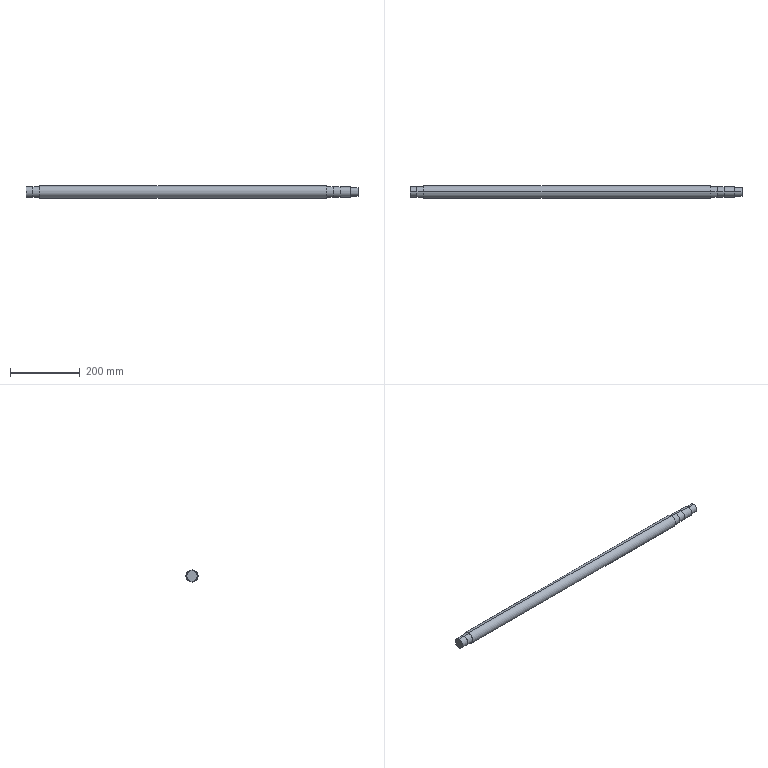Part | SolidWorks | features ICE 6, Extrusion 1, HoleWzd 1, MirrorPattern 1 | 1 solid | 41 faces | box 949 x 35 x 35 mm | volume 873181 mm3 | cylinder 22 | plane 17 | cone 2 | commonest cylinder face diameters 10 x4 30 x4 31 x4 6.8 x2 8 x2 25 x2
STEP:
#1=CARTESIAN_POINT('',(480.,0.,3.4));
#2=VERTEX_POINT('',#1);
#3=CARTESIAN_POINT('',(480.,0.,-3.4));
#4=VERTEX_POINT('',#3);
#5=CARTESIAN_POINT('',(480.,0.,0.));
#6=DIRECTION('',(1.,0.,0.));
#7=DIRECTION('',(0.,0.,-1.));
#8=AXIS2_PLACEMENT_3D('',#5,#6,#7);
#9=CIRCLE('',#8,3.4);
#10=EDGE_CURVE('',#2,#4,#9,.T.);
#11=ORIENTED_EDGE('',*,*,#10,.F.);
#12=CARTESIAN_POINT('',(500.,0.,3.4));
#13=VERTEX_POINT('',#12);
#14=CARTESIAN_POINT('',(500.,0.,3.4));
#15=DIRECTION('',(1.,0.,0.));
#16=VECTOR('',#15,1000.);
#17=LINE('',#14,#16);
#18=EDGE_CURVE('',#2,#13,#17,.T.);
#19=ORIENTED_EDGE('',*,*,#18,.T.);
#20=CARTESIAN_POINT('',(500.,0.,-3.4));
#21=VERTEX_POINT('',#20);
#22=CARTESIAN_POINT('',(500.,0.,0.));
#23=DIRECTION('',(1.,0.,0.));
#24=DIRECTION('',(0.,0.,-1.));
#25=AXIS2_PLACEMENT_3D('',#22,#23,#24);
#26=CIRCLE('',#25,3.4);
#27=EDGE_CURVE('',#13,#21,#26,.T.);
#28=ORIENTED_EDGE('',*,*,#27,.T.);
#29=CARTESIAN_POINT('',(500.,0.,-3.4));
#30=DIRECTION('',(1.,0.,0.));
#31=VECTOR('',#30,1000.);
#32=LINE('',#29,#31);
#33=EDGE_CURVE('',#4,#21,#32,.T.);
#34=ORIENTED_EDGE('',*,*,#33,.F.);
#35=EDGE_LOOP('',(#11,#19,#28,#34));
#36=FACE_OUTER_BOUND('',#35,.T.);
#37=CARTESIAN_POINT('',(500.,0.,0.));
#38=DIRECTION('',(1.,0.,0.));
#39=DIRECTION('',(0.,0.,-1.));
#40=AXIS2_PLACEMENT_3D('',#37,#38,#39);
#41=CYLINDRICAL_SURFACE('',#40,3.4);
#42=ADVANCED_FACE('',(#36),#41,.F.);
#43=CARTESIAN_POINT('',(477.957,0.,0.));
#44=VERTEX_POINT('',#43);
#45=CARTESIAN_POINT('',(480.,0.,-3.4));
#46=DIRECTION('',(0.515,0.,-0.8572));
#47=VECTOR('',#46,1000.);
#48=LINE('',#45,#47);
#49=EDGE_CURVE('',#44,#4,#48,.T.);
#50=ORIENTED_EDGE('',*,*,#49,.F.);
#51=CARTESIAN_POINT('',(480.,0.,3.4));
#52=DIRECTION('',(0.515,0.,0.8572));
#53=VECTOR('',#52,1000.);
#54=LINE('',#51,#53);
#55=EDGE_CURVE('',#44,#2,#54,.T.);
#56=ORIENTED_EDGE('',*,*,#55,.T.);
#57=ORIENTED_EDGE('',*,*,#10,.T.);
#58=EDGE_LOOP('',(#50,#56,#57));
#59=FACE_OUTER_BOUND('',#58,.T.);
#60=CARTESIAN_POINT('',(480.,0.,0.));
#61=DIRECTION('',(1.,0.,0.));
#62=DIRECTION('',(0.,0.,-1.));
#63=AXIS2_PLACEMENT_3D('',#60,#61,#62);
#64=CONICAL_SURFACE('',#63,3.4,1.03);
#65=ADVANCED_FACE('',(#59),#64,.F.);
#66=CARTESIAN_POINT('',(-449.,0.,-15.));
#67=VERTEX_POINT('',#66);
#68=CARTESIAN_POINT('',(-449.,0.,15.));
#69=VERTEX_POINT('',#68);
#70=CARTESIAN_POINT('',(-449.,0.,0.));
#71=DIRECTION('',(1.,0.,0.));
#72=DIRECTION('',(0.,0.,-1.));
#73=AXIS2_PLACEMENT_3D('',#70,#71,#72);
#74=CIRCLE('',#73,15.);
#75=EDGE_CURVE('',#67,#69,#74,.T.);
#76=ORIENTED_EDGE('',*,*,#75,.T.);
#77=CARTESIAN_POINT('',(-429.,0.,15.));
#78=VERTEX_POINT('',#77);
#79=CARTESIAN_POINT('',(-449.,0.,15.));
#80=DIRECTION('',(1.,0.,0.));
#81=VECTOR('',#80,1000.);
#82=LINE('',#79,#81);
#83=EDGE_CURVE('',#69,#78,#82,.T.);
#84=ORIENTED_EDGE('',*,*,#83,.T.);
#85=CARTESIAN_POINT('',(-429.,0.,-15.));
#86=VERTEX_POINT('',#85);
#87=CARTESIAN_POINT('',(-429.,0.,0.));
#88=DIRECTION('',(-1.,0.,0.));
#89=DIRECTION('',(0.,0.,1.));
#90=AXIS2_PLACEMENT_3D('',#87,#88,#89);
#91=CIRCLE('',#90,15.);
#92=EDGE_CURVE('',#78,#86,#91,.T.);
#93=ORIENTED_EDGE('',*,*,#92,.T.);
#94=CARTESIAN_POINT('',(-449.,0.,-15.));
#95=DIRECTION('',(1.,0.,0.));
#96=VECTOR('',#95,1000.);
#97=LINE('',#94,#96);
#98=EDGE_CURVE('',#67,#86,#97,.T.);
#99=ORIENTED_EDGE('',*,*,#98,.F.);
#100=EDGE_LOOP('',(#76,#84,#93,#99));
#101=FACE_OUTER_BOUND('',#100,.T.);
#102=CARTESIAN_POINT('',(-449.,0.,0.));
#103=DIRECTION('',(1.,0.,0.));
#104=DIRECTION('',(0.,0.,-1.));
#105=AXIS2_PLACEMENT_3D('',#102,#103,#104);
#106=CYLINDRICAL_SURFACE('',#105,15.);
#107=ADVANCED_FACE('',(#101),#106,.T.);
#108=CARTESIAN_POINT('',(-422.,14.671,-5.));
#109=VERTEX_POINT('',#108);
#110=CARTESIAN_POINT('',(-422.,14.671,5.));
#111=VERTEX_POINT('',#110);
#112=CARTESIAN_POINT('',(-422.,14.671,-5.));
#113=CARTESIAN_POINT('',(-422.333,14.671,-5.));
#114=CARTESIAN_POINT('',(-422.659,14.683,-4.967));
#115=CARTESIAN_POINT('',(-423.301,14.725,-4.839));
#116=CARTESIAN_POINT('',(-423.62,14.757,-4.742));
#117=CARTESIAN_POINT('',(-424.224,14.836,-4.49));
#118=CARTESIAN_POINT('',(-424.51,14.882,-4.337));
#119=CARTESIAN_POINT('',(-425.052,14.983,-3.974));
#120=CARTESIAN_POINT('',(-425.306,15.038,-3.765));
#121=CARTESIAN_POINT('',(-425.764,15.145,-3.307));
#122=CARTESIAN_POINT('',(-425.97,15.198,-3.057));
#123=CARTESIAN_POINT('',(-426.336,15.298,-2.511));
#124=CARTESIAN_POINT('',(-426.49,15.343,-2.224));
#125=CARTESIAN_POINT('',(-426.678,15.399,-1.773));
#126=CARTESIAN_POINT('',(-426.733,15.416,-1.62));
#127=CARTESIAN_POINT('',(-426.829,15.446,-1.306));
#128=CARTESIAN_POINT('',(-426.87,15.459,-1.144));
#129=CARTESIAN_POINT('',(-426.967,15.489,-0.6596));
#130=CARTESIAN_POINT('',(-427.,15.5,-0.3337));
#131=CARTESIAN_POINT('',(-427.,15.5,0.3234));
#132=CARTESIAN_POINT('',(-426.967,15.489,0.6571));
#133=CARTESIAN_POINT('',(-426.839,15.449,1.3));
#134=CARTESIAN_POINT('',(-426.744,15.419,1.613));
#135=CARTESIAN_POINT('',(-426.492,15.343,2.221));
#136=CARTESIAN_POINT('',(-426.336,15.298,2.51));
#137=CARTESIAN_POINT('',(-425.975,15.199,3.05));
#138=CARTESIAN_POINT('',(-425.767,15.146,3.304));
#139=CARTESIAN_POINT('',(-425.306,15.038,3.765));
#140=CARTESIAN_POINT('',(-425.056,14.984,3.97));
#141=CARTESIAN_POINT('',(-424.517,14.883,4.333));
#142=CARTESIAN_POINT('',(-424.225,14.836,4.49));
#143=CARTESIAN_POINT('',(-423.623,14.758,4.74));
#144=CARTESIAN_POINT('',(-423.311,14.726,4.836));
#145=CARTESIAN_POINT('',(-422.665,14.683,4.967));
#146=CARTESIAN_POINT('',(-422.333,14.671,5.));
#147=CARTESIAN_POINT('',(-422.,14.671,5.));
#148=B_SPLINE_CURVE_WITH_KNOTS('',3,(#112,#113,#114,#115,#116,#117,#118,#119,#120,#121,#122,#123,#124,#125,#126,#127,#128,#129,#130,#131,#132,#133,#134,#135,#136,#137,#138,#139,#140,#141,#142,#143,#144,#145,#146,#147),.UNSPECIFIED.,.F.,.F.,(4,2,2,2,2,2,2,2,2,2,2,2,2,2,2,2,2,4),(0.,0.0009833,0.001967,0.00295,0.003933,0.004916,0.0059,0.006391,0.006883,0.007866,0.008849,0.009833,0.01082,0.0118,0.01278,0.01377,0.01475,0.01573),.UNSPECIFIED.);
#149=EDGE_CURVE('',#109,#111,#148,.T.);
#150=ORIENTED_EDGE('',*,*,#149,.F.);
#151=CARTESIAN_POINT('',(-418.,14.671,-5.));
#152=VERTEX_POINT('',#151);
#153=CARTESIAN_POINT('',(-429.,14.671,-5.));
#154=DIRECTION('',(-1.,0.,0.));
#155=VECTOR('',#154,1000.);
#156=LINE('',#153,#155);
#157=EDGE_CURVE('',#152,#109,#156,.T.);
#158=ORIENTED_EDGE('',*,*,#157,.F.);
#159=CARTESIAN_POINT('',(-418.,14.671,5.));
#160=VERTEX_POINT('',#159);
#161=CARTESIAN_POINT('',(-418.,14.671,5.));
#162=CARTESIAN_POINT('',(-417.667,14.671,5.));
#163=CARTESIAN_POINT('',(-417.34,14.683,4.967));
#164=CARTESIAN_POINT('',(-416.698,14.726,4.839));
#165=CARTESIAN_POINT('',(-416.38,14.758,4.741));
#166=CARTESIAN_POINT('',(-415.775,14.836,4.49));
#167=CARTESIAN_POINT('',(-415.489,14.882,4.336));
#168=CARTESIAN_POINT('',(-414.947,14.983,3.973));
#169=CARTESIAN_POINT('',(-414.693,15.038,3.764));
#170=CARTESIAN_POINT('',(-414.235,15.145,3.306));
#171=CARTESIAN_POINT('',(-414.029,15.198,3.056));
#172=CARTESIAN_POINT('',(-413.663,15.298,2.509));
#173=CARTESIAN_POINT('',(-413.509,15.343,2.222));
#174=CARTESIAN_POINT('',(-413.321,15.399,1.771));
#175=CARTESIAN_POINT('',(-413.266,15.416,1.618));
#176=CARTESIAN_POINT('',(-413.17,15.446,1.303));
#177=CARTESIAN_POINT('',(-413.129,15.459,1.142));
#178=CARTESIAN_POINT('',(-413.032,15.489,0.6569));
#179=CARTESIAN_POINT('',(-413.,15.5,0.3309));
#180=CARTESIAN_POINT('',(-413.,15.5,-0.3264));
#181=CARTESIAN_POINT('',(-413.033,15.489,-0.6603));
#182=CARTESIAN_POINT('',(-413.162,15.448,-1.304));
#183=CARTESIAN_POINT('',(-413.257,15.419,-1.616));
#184=CARTESIAN_POINT('',(-413.51,15.343,-2.225));
#185=CARTESIAN_POINT('',(-413.666,15.297,-2.514));
#186=CARTESIAN_POINT('',(-414.027,15.199,-3.053));
#187=CARTESIAN_POINT('',(-414.236,15.145,-3.307));
#188=CARTESIAN_POINT('',(-414.697,15.037,-3.768));
#189=CARTESIAN_POINT('',(-414.947,14.983,-3.973));
#190=CARTESIAN_POINT('',(-415.487,14.883,-4.335));
#191=CARTESIAN_POINT('',(-415.78,14.835,-4.492));
#192=CARTESIAN_POINT('',(-416.382,14.757,-4.742));
#193=CARTESIAN_POINT('',(-416.694,14.726,-4.838));
#194=CARTESIAN_POINT('',(-417.179,14.693,-4.935));
#195=CARTESIAN_POINT('',(-417.344,14.685,-4.96));
#196=CARTESIAN_POINT('',(-417.672,14.674,-4.992));
#197=CARTESIAN_POINT('',(-417.836,14.671,-5.));
#198=CARTESIAN_POINT('',(-418.,14.671,-5.));
#199=B_SPLINE_CURVE_WITH_KNOTS('',3,(#161,#162,#163,#164,#165,#166,#167,#168,#169,#170,#171,#172,#173,#174,#175,#176,#177,#178,#179,#180,#181,#182,#183,#184,#185,#186,#187,#188,#189,#190,#191,#192,#193,#194,#195,#196,#197,#198),.UNSPECIFIED.,.F.,.F.,(4,2,2,2,2,2,2,2,2,2,2,2,2,2,2,2,2,2,4),(0.,0.0009836,0.001967,0.002951,0.003934,0.004918,0.005902,0.006394,0.006885,0.007869,0.008853,0.009836,0.01082,0.0118,0.01279,0.01377,0.01475,0.01525,0.01574),.UNSPECIFIED.);
#200=EDGE_CURVE('',#160,#152,#199,.T.);
#201=ORIENTED_EDGE('',*,*,#200,.F.);
#202=CARTESIAN_POINT('',(-429.,14.671,5.));
#203=DIRECTION('',(1.,0.,0.));
#204=VECTOR('',#203,1000.);
#205=LINE('',#202,#204);
#206=EDGE_CURVE('',#111,#160,#205,.T.);
#207=ORIENTED_EDGE('',*,*,#206,.F.);
#208=EDGE_LOOP('',(#150,#158,#201,#207));
#209=FACE_BOUND('',#208,.T.);
#210=CARTESIAN_POINT('',(-429.,0.,-15.5));
#211=VERTEX_POINT('',#210);
#212=CARTESIAN_POINT('',(-429.,0.,15.5));
#213=VERTEX_POINT('',#212);
#214=CARTESIAN_POINT('',(-429.,0.,0.));
#215=DIRECTION('',(1.,0.,0.));
#216=DIRECTION('',(0.,0.,-1.));
#217=AXIS2_PLACEMENT_3D('',#214,#215,#216);
#218=CIRCLE('',#217,15.5);
#219=EDGE_CURVE('',#211,#213,#218,.T.);
#220=ORIENTED_EDGE('',*,*,#219,.T.);
#221=CARTESIAN_POINT('',(-410.,0.,15.5));
#222=VERTEX_POINT('',#221);
#223=CARTESIAN_POINT('',(-429.,0.,15.5));
#224=DIRECTION('',(1.,0.,0.));
#225=VECTOR('',#224,1000.);
#226=LINE('',#223,#225);
#227=EDGE_CURVE('',#213,#222,#226,.T.);
#228=ORIENTED_EDGE('',*,*,#227,.T.);
#229=CARTESIAN_POINT('',(-410.,0.,-15.5));
#230=VERTEX_POINT('',#229);
#231=CARTESIAN_POINT('',(-410.,0.,0.));
#232=DIRECTION('',(1.,0.,0.));
#233=DIRECTION('',(0.,0.,-1.));
#234=AXIS2_PLACEMENT_3D('',#231,#232,#233);
#235=CIRCLE('',#234,15.5);
#236=EDGE_CURVE('',#230,#222,#235,.T.);
#237=ORIENTED_EDGE('',*,*,#236,.F.);
#238=CARTESIAN_POINT('',(-429.,0.,-15.5));
#239=DIRECTION('',(1.,0.,0.));
#240=VECTOR('',#239,1000.);
#241=LINE('',#238,#240);
#242=EDGE_CURVE('',#211,#230,#241,.T.);
#243=ORIENTED_EDGE('',*,*,#242,.F.);
#244=EDGE_LOOP('',(#220,#228,#237,#243));
#245=FACE_OUTER_BOUND('',#244,.T.);
#246=CARTESIAN_POINT('',(-429.,0.,0.));
#247=DIRECTION('',(1.,0.,0.));
#248=DIRECTION('',(0.,0.,-1.));
#249=AXIS2_PLACEMENT_3D('',#246,#247,#248);
#250=CYLINDRICAL_SURFACE('',#249,15.5);
#251=ADVANCED_FACE('',(#209,#245),#250,.T.);
#252=CARTESIAN_POINT('',(494.,11.843,4.));
#253=VERTEX_POINT('',#252);
#254=CARTESIAN_POINT('',(484.,11.843,4.));
#255=VERTEX_POINT('',#254);
#256=CARTESIAN_POINT('',(500.,11.843,4.));
#257=DIRECTION('',(-1.,0.,0.));
#258=VECTOR('',#257,1000.);
#259=LINE('',#256,#258);
#260=EDGE_CURVE('',#253,#255,#259,.T.);
#261=ORIENTED_EDGE('',*,*,#260,.T.);
#262=CARTESIAN_POINT('',(484.,11.843,-4.));
#263=VERTEX_POINT('',#262);
#264=CARTESIAN_POINT('',(484.,11.843,4.));
#265=CARTESIAN_POINT('',(483.734,11.843,4.));
#266=CARTESIAN_POINT('',(483.473,11.852,3.974));
#267=CARTESIAN_POINT('',(482.959,11.886,3.871));
#268=CARTESIAN_POINT('',(482.704,11.911,3.793));
#269=CARTESIAN_POINT('',(482.221,11.973,3.592));
#270=CARTESIAN_POINT('',(481.992,12.01,3.469));
#271=CARTESIAN_POINT('',(481.559,12.09,3.179));
#272=CARTESIAN_POINT('',(481.355,12.133,3.012));
#273=CARTESIAN_POINT('',(480.989,12.218,2.646));
#274=CARTESIAN_POINT('',(480.824,12.26,2.445));
#275=CARTESIAN_POINT('',(480.531,12.34,2.009));
#276=CARTESIAN_POINT('',(480.408,12.375,1.779));
#277=CARTESIAN_POINT('',(480.208,12.435,1.299));
#278=CARTESIAN_POINT('',(480.13,12.459,1.045));
#279=CARTESIAN_POINT('',(480.026,12.492,0.5276));
#280=CARTESIAN_POINT('',(480.,12.5,0.2669));
#281=CARTESIAN_POINT('',(480.,12.5,-0.2587));
#282=CARTESIAN_POINT('',(480.026,12.492,-0.5256));
#283=CARTESIAN_POINT('',(480.129,12.459,-1.04));
#284=CARTESIAN_POINT('',(480.205,12.436,-1.29));
#285=CARTESIAN_POINT('',(480.407,12.375,-1.777));
#286=CARTESIAN_POINT('',(480.531,12.34,-2.008));
#287=CARTESIAN_POINT('',(480.82,12.262,-2.44));
#288=CARTESIAN_POINT('',(480.987,12.219,-2.643));
#289=CARTESIAN_POINT('',(481.355,12.133,-3.012));
#290=CARTESIAN_POINT('',(481.555,12.091,-3.176));
#291=CARTESIAN_POINT('',(481.987,12.011,-3.466));
#292=CARTESIAN_POINT('',(482.22,11.973,-3.592));
#293=CARTESIAN_POINT('',(482.702,11.911,-3.792));
#294=CARTESIAN_POINT('',(482.951,11.886,-3.869));
#295=CARTESIAN_POINT('',(483.468,11.852,-3.973));
#296=CARTESIAN_POINT('',(483.734,11.843,-4.));
#297=CARTESIAN_POINT('',(484.,11.843,-4.));
#298=B_SPLINE_CURVE_WITH_KNOTS('',3,(#264,#265,#266,#267,#268,#269,#270,#271,#272,#273,#274,#275,#276,#277,#278,#279,#280,#281,#282,#283,#284,#285,#286,#287,#288,#289,#290,#291,#292,#293,#294,#295,#296,#297),.UNSPECIFIED.,.F.,.F.,(4,2,2,2,2,2,2,2,2,2,2,2,2,2,2,2,4),(0.,0.0007865,0.001573,0.00236,0.003146,0.003933,0.004719,0.005506,0.006292,0.007079,0.007865,0.008652,0.009438,0.01022,0.01101,0.0118,0.01258),.UNSPECIFIED.);
#299=EDGE_CURVE('',#255,#263,#298,.T.);
#300=ORIENTED_EDGE('',*,*,#299,.T.);
#301=CARTESIAN_POINT('',(494.,11.843,-4.));
#302=VERTEX_POINT('',#301);
#303=CARTESIAN_POINT('',(500.,11.843,-4.));
#304=DIRECTION('',(1.,0.,0.));
#305=VECTOR('',#304,1000.);
#306=LINE('',#303,#305);
#307=EDGE_CURVE('',#263,#302,#306,.T.);
#308=ORIENTED_EDGE('',*,*,#307,.T.);
#309=CARTESIAN_POINT('',(494.,11.843,-4.));
#310=CARTESIAN_POINT('',(494.266,11.843,-4.));
#311=CARTESIAN_POINT('',(494.527,11.852,-3.974));
#312=CARTESIAN_POINT('',(495.041,11.886,-3.871));
#313=CARTESIAN_POINT('',(495.296,11.911,-3.793));
#314=CARTESIAN_POINT('',(495.779,11.973,-3.592));
#315=CARTESIAN_POINT('',(496.008,12.01,-3.469));
#316=CARTESIAN_POINT('',(496.441,12.09,-3.179));
#317=CARTESIAN_POINT('',(496.645,12.133,-3.012));
#318=CARTESIAN_POINT('',(497.011,12.218,-2.646));
#319=CARTESIAN_POINT('',(497.176,12.26,-2.445));
#320=CARTESIAN_POINT('',(497.469,12.34,-2.009));
#321=CARTESIAN_POINT('',(497.592,12.375,-1.779));
#322=CARTESIAN_POINT('',(497.792,12.435,-1.299));
#323=CARTESIAN_POINT('',(497.87,12.459,-1.045));
#324=CARTESIAN_POINT('',(497.974,12.492,-0.5276));
#325=CARTESIAN_POINT('',(498.,12.5,-0.2669));
#326=CARTESIAN_POINT('',(498.,12.5,0.2587));
#327=CARTESIAN_POINT('',(497.974,12.492,0.5256));
#328=CARTESIAN_POINT('',(497.871,12.459,1.04));
#329=CARTESIAN_POINT('',(497.795,12.436,1.29));
#330=CARTESIAN_POINT('',(497.593,12.375,1.777));
#331=CARTESIAN_POINT('',(497.469,12.34,2.008));
#332=CARTESIAN_POINT('',(497.18,12.262,2.44));
#333=CARTESIAN_POINT('',(497.013,12.219,2.643));
#334=CARTESIAN_POINT('',(496.645,12.133,3.012));
#335=CARTESIAN_POINT('',(496.445,12.091,3.176));
#336=CARTESIAN_POINT('',(496.013,12.011,3.466));
#337=CARTESIAN_POINT('',(495.78,11.973,3.592));
#338=CARTESIAN_POINT('',(495.298,11.911,3.792));
#339=CARTESIAN_POINT('',(495.049,11.886,3.869));
#340=CARTESIAN_POINT('',(494.532,11.852,3.973));
#341=CARTESIAN_POINT('',(494.266,11.843,4.));
#342=CARTESIAN_POINT('',(494.,11.843,4.));
#343=B_SPLINE_CURVE_WITH_KNOTS('',3,(#309,#310,#311,#312,#313,#314,#315,#316,#317,#318,#319,#320,#321,#322,#323,#324,#325,#326,#327,#328,#329,#330,#331,#332,#333,#334,#335,#336,#337,#338,#339,#340,#341,#342),.UNSPECIFIED.,.F.,.F.,(4,2,2,2,2,2,2,2,2,2,2,2,2,2,2,2,4),(0.,0.0007865,0.001573,0.00236,0.003146,0.003933,0.004719,0.005506,0.006292,0.007079,0.007865,0.008652,0.009438,0.01022,0.01101,0.0118,0.01258),.UNSPECIFIED.);
#344=EDGE_CURVE('',#302,#253,#343,.T.);
#345=ORIENTED_EDGE('',*,*,#344,.T.);
#346=EDGE_LOOP('',(#261,#300,#308,#345));
#347=FACE_BOUND('',#346,.T.);
#348=CARTESIAN_POINT('',(500.,0.,-12.5));
#349=VERTEX_POINT('',#348);
#350=CARTESIAN_POINT('',(500.,0.,12.5));
#351=VERTEX_POINT('',#350);
#352=CARTESIAN_POINT('',(500.,0.,0.));
#353=DIRECTION('',(1.,0.,0.));
#354=DIRECTION('',(0.,0.,-1.));
#355=AXIS2_PLACEMENT_3D('',#352,#353,#354);
#356=CIRCLE('',#355,12.5);
#357=EDGE_CURVE('',#349,#351,#356,.T.);
#358=ORIENTED_EDGE('',*,*,#357,.F.);
#359=CARTESIAN_POINT('',(478.,0.,-12.5));
#360=VERTEX_POINT('',#359);
#361=CARTESIAN_POINT('',(500.,0.,-12.5));
#362=DIRECTION('',(-1.,0.,0.));
#363=VECTOR('',#362,1000.);
#364=LINE('',#361,#363);
#365=EDGE_CURVE('',#349,#360,#364,.T.);
#366=ORIENTED_EDGE('',*,*,#365,.T.);
#367=CARTESIAN_POINT('',(478.,0.,12.5));
#368=VERTEX_POINT('',#367);
#369=CARTESIAN_POINT('',(478.,0.,0.));
#370=DIRECTION('',(1.,0.,0.));
#371=DIRECTION('',(0.,0.,-1.));
#372=AXIS2_PLACEMENT_3D('',#369,#370,#371);
#373=CIRCLE('',#372,12.5);
#374=EDGE_CURVE('',#360,#368,#373,.T.);
#375=ORIENTED_EDGE('',*,*,#374,.T.);
#376=CARTESIAN_POINT('',(500.,0.,12.5));
#377=DIRECTION('',(-1.,0.,0.));
#378=VECTOR('',#377,1000.);
#379=LINE('',#376,#378);
#380=EDGE_CURVE('',#351,#368,#379,.T.);
#381=ORIENTED_EDGE('',*,*,#380,.F.);
#382=EDGE_LOOP('',(#358,#366,#375,#381));
#383=FACE_OUTER_BOUND('',#382,.T.);
#384=CARTESIAN_POINT('',(500.,0.,0.));
#385=DIRECTION('',(-1.,0.,0.));
#386=DIRECTION('',(0.,0.,1.));
#387=AXIS2_PLACEMENT_3D('',#384,#385,#386);
#388=CYLINDRICAL_SURFACE('',#387,12.5);
#389=ADVANCED_FACE('',(#347,#383),#388,.T.);
#390=CARTESIAN_POINT('',(478.,0.,-14.5));
#391=VERTEX_POINT('',#390);
#392=CARTESIAN_POINT('',(478.,0.,14.5));
#393=VERTEX_POINT('',#392);
#394=CARTESIAN_POINT('',(478.,0.,0.));
#395=DIRECTION('',(1.,0.,0.));
#396=DIRECTION('',(0.,0.,-1.));
#397=AXIS2_PLACEMENT_3D('',#394,#395,#396);
#398=CIRCLE('',#397,14.5);
#399=EDGE_CURVE('',#391,#393,#398,.T.);
#400=ORIENTED_EDGE('',*,*,#399,.F.);
#401=CARTESIAN_POINT('',(449.,0.,-14.5));
#402=VERTEX_POINT('',#401);
#403=CARTESIAN_POINT('',(478.,0.,-14.5));
#404=DIRECTION('',(-1.,0.,0.));
#405=VECTOR('',#404,1000.);
#406=LINE('',#403,#405);
#407=EDGE_CURVE('',#391,#402,#406,.T.);
#408=ORIENTED_EDGE('',*,*,#407,.T.);
#409=CARTESIAN_POINT('',(449.,0.,14.5));
#410=VERTEX_POINT('',#409);
#411=CARTESIAN_POINT('',(449.,0.,0.));
#412=DIRECTION('',(1.,0.,0.));
#413=DIRECTION('',(0.,0.,-1.));
#414=AXIS2_PLACEMENT_3D('',#411,#412,#413);
#415=CIRCLE('',#414,14.5);
#416=EDGE_CURVE('',#402,#410,#415,.T.);
#417=ORIENTED_EDGE('',*,*,#416,.T.);
#418=CARTESIAN_POINT('',(478.,0.,14.5));
#419=DIRECTION('',(-1.,0.,0.));
#420=VECTOR('',#419,1000.);
#421=LINE('',#418,#420);
#422=EDGE_CURVE('',#393,#410,#421,.T.);
#423=ORIENTED_EDGE('',*,*,#422,.F.);
#424=EDGE_LOOP('',(#400,#408,#417,#423));
#425=FACE_OUTER_BOUND('',#424,.T.);
#426=CARTESIAN_POINT('',(478.,0.,0.));
#427=DIRECTION('',(-1.,0.,0.));
#428=DIRECTION('',(0.,0.,1.));
#429=AXIS2_PLACEMENT_3D('',#426,#427,#428);
#430=CYLINDRICAL_SURFACE('',#429,14.5);
#431=ADVANCED_FACE('',(#425),#430,.T.);
#432=CARTESIAN_POINT('',(449.,0.,-15.));
#433=VERTEX_POINT('',#432);
#434=CARTESIAN_POINT('',(449.,0.,15.));
#435=VERTEX_POINT('',#434);
#436=CARTESIAN_POINT('',(449.,0.,0.));
#437=DIRECTION('',(1.,0.,0.));
#438=DIRECTION('',(0.,0.,-1.));
#439=AXIS2_PLACEMENT_3D('',#436,#437,#438);
#440=CIRCLE('',#439,15.);
#441=EDGE_CURVE('',#433,#435,#440,.T.);
#442=ORIENTED_EDGE('',*,*,#441,.F.);
#443=CARTESIAN_POINT('',(429.,0.,-15.));
#444=VERTEX_POINT('',#443);
#445=CARTESIAN_POINT('',(449.,0.,-15.));
#446=DIRECTION('',(-1.,0.,0.));
#447=VECTOR('',#446,1000.);
#448=LINE('',#445,#447);
#449=EDGE_CURVE('',#433,#444,#448,.T.);
#450=ORIENTED_EDGE('',*,*,#449,.T.);
#451=CARTESIAN_POINT('',(429.,0.,15.));
#452=VERTEX_POINT('',#451);
#453=CARTESIAN_POINT('',(429.,0.,0.));
#454=DIRECTION('',(1.,0.,0.));
#455=DIRECTION('',(0.,0.,-1.));
#456=AXIS2_PLACEMENT_3D('',#453,#454,#455);
#457=CIRCLE('',#456,15.);
#458=EDGE_CURVE('',#444,#452,#457,.T.);
#459=ORIENTED_EDGE('',*,*,#458,.T.);
#460=CARTESIAN_POINT('',(449.,0.,15.));
#461=DIRECTION('',(-1.,0.,0.));
#462=VECTOR('',#461,1000.);
#463=LINE('',#460,#462);
#464=EDGE_CURVE('',#435,#452,#463,.T.);
#465=ORIENTED_EDGE('',*,*,#464,.F.);
#466=EDGE_LOOP('',(#442,#450,#459,#465));
#467=FACE_OUTER_BOUND('',#466,.T.);
#468=CARTESIAN_POINT('',(449.,0.,0.));
#469=DIRECTION('',(-1.,0.,0.));
#470=DIRECTION('',(0.,0.,1.));
#471=AXIS2_PLACEMENT_3D('',#468,#469,#470);
#472=CYLINDRICAL_SURFACE('',#471,15.);
#473=ADVANCED_FACE('',(#467),#472,.T.);
#474=CARTESIAN_POINT('',(422.,14.671,5.));
#475=VERTEX_POINT('',#474);
#476=CARTESIAN_POINT('',(418.,14.671,5.));
#477=VERTEX_POINT('',#476);
#478=CARTESIAN_POINT('',(429.,14.671,5.));
#479=DIRECTION('',(-1.,0.,0.));
#480=VECTOR('',#479,1000.);
#481=LINE('',#478,#480);
#482=EDGE_CURVE('',#475,#477,#481,.T.);
#483=ORIENTED_EDGE('',*,*,#482,.T.);
#484=CARTESIAN_POINT('',(418.,14.671,-5.));
#485=VERTEX_POINT('',#484);
#486=CARTESIAN_POINT('',(418.,14.671,5.));
#487=CARTESIAN_POINT('',(417.667,14.671,5.));
#488=CARTESIAN_POINT('',(417.341,14.683,4.967));
#489=CARTESIAN_POINT('',(416.699,14.725,4.839));
#490=CARTESIAN_POINT('',(416.38,14.757,4.742));
#491=CARTESIAN_POINT('',(415.776,14.836,4.49));
#492=CARTESIAN_POINT('',(415.49,14.882,4.337));
#493=CARTESIAN_POINT('',(414.948,14.983,3.974));
#494=CARTESIAN_POINT('',(414.694,15.038,3.765));
#495=CARTESIAN_POINT('',(414.236,15.145,3.307));
#496=CARTESIAN_POINT('',(414.03,15.198,3.057));
#497=CARTESIAN_POINT('',(413.664,15.298,2.511));
#498=CARTESIAN_POINT('',(413.51,15.343,2.224));
#499=CARTESIAN_POINT('',(413.322,15.399,1.773));
#500=CARTESIAN_POINT('',(413.267,15.416,1.62));
#501=CARTESIAN_POINT('',(413.171,15.446,1.306));
#502=CARTESIAN_POINT('',(413.13,15.459,1.144));
#503=CARTESIAN_POINT('',(413.033,15.489,0.6596));
#504=CARTESIAN_POINT('',(413.,15.5,0.3337));
#505=CARTESIAN_POINT('',(413.,15.5,-0.3234));
#506=CARTESIAN_POINT('',(413.033,15.489,-0.6571));
#507=CARTESIAN_POINT('',(413.161,15.449,-1.3));
#508=CARTESIAN_POINT('',(413.256,15.419,-1.613));
#509=CARTESIAN_POINT('',(413.508,15.343,-2.221));
#510=CARTESIAN_POINT('',(413.664,15.298,-2.51));
#511=CARTESIAN_POINT('',(414.025,15.199,-3.05));
#512=CARTESIAN_POINT('',(414.233,15.146,-3.304));
#513=CARTESIAN_POINT('',(414.694,15.038,-3.765));
#514=CARTESIAN_POINT('',(414.944,14.984,-3.97));
#515=CARTESIAN_POINT('',(415.483,14.883,-4.333));
#516=CARTESIAN_POINT('',(415.775,14.836,-4.49));
#517=CARTESIAN_POINT('',(416.377,14.758,-4.74));
#518=CARTESIAN_POINT('',(416.689,14.726,-4.836));
#519=CARTESIAN_POINT('',(417.335,14.683,-4.967));
#520=CARTESIAN_POINT('',(417.667,14.671,-5.));
#521=CARTESIAN_POINT('',(418.,14.671,-5.));
#522=B_SPLINE_CURVE_WITH_KNOTS('',3,(#486,#487,#488,#489,#490,#491,#492,#493,#494,#495,#496,#497,#498,#499,#500,#501,#502,#503,#504,#505,#506,#507,#508,#509,#510,#511,#512,#513,#514,#515,#516,#517,#518,#519,#520,#521),.UNSPECIFIED.,.F.,.F.,(4,2,2,2,2,2,2,2,2,2,2,2,2,2,2,2,2,4),(0.,0.0009833,0.001967,0.00295,0.003933,0.004916,0.0059,0.006391,0.006883,0.007866,0.008849,0.009833,0.01082,0.0118,0.01278,0.01377,0.01475,0.01573),.UNSPECIFIED.);
#523=EDGE_CURVE('',#477,#485,#522,.T.);
#524=ORIENTED_EDGE('',*,*,#523,.T.);
#525=CARTESIAN_POINT('',(422.,14.671,-5.));
#526=VERTEX_POINT('',#525);
#527=CARTESIAN_POINT('',(429.,14.671,-5.));
#528=DIRECTION('',(1.,0.,0.));
#529=VECTOR('',#528,1000.);
#530=LINE('',#527,#529);
#531=EDGE_CURVE('',#485,#526,#530,.T.);
#532=ORIENTED_EDGE('',*,*,#531,.T.);
#533=CARTESIAN_POINT('',(422.,14.671,-5.));
#534=CARTESIAN_POINT('',(422.328,14.671,-5.));
#535=CARTESIAN_POINT('',(422.657,14.683,-4.968));
#536=CARTESIAN_POINT('',(423.306,14.726,-4.838));
#537=CARTESIAN_POINT('',(423.619,14.757,-4.742));
#538=CARTESIAN_POINT('',(424.221,14.836,-4.491));
#539=CARTESIAN_POINT('',(424.514,14.883,-4.334));
#540=CARTESIAN_POINT('',(425.054,14.984,-3.972));
#541=CARTESIAN_POINT('',(425.304,15.037,-3.767));
#542=CARTESIAN_POINT('',(425.766,15.145,-3.305));
#543=CARTESIAN_POINT('',(425.974,15.199,-3.052));
#544=CARTESIAN_POINT('',(426.335,15.297,-2.513));
#545=CARTESIAN_POINT('',(426.49,15.343,-2.225));
#546=CARTESIAN_POINT('',(426.743,15.419,-1.616));
#547=CARTESIAN_POINT('',(426.838,15.448,-1.304));
#548=CARTESIAN_POINT('',(426.967,15.489,-0.6623));
#549=CARTESIAN_POINT('',(427.,15.5,-0.3291));
#550=CARTESIAN_POINT('',(427.,15.5,0.3298));
#551=CARTESIAN_POINT('',(426.968,15.489,0.656));
#552=CARTESIAN_POINT('',(426.871,15.459,1.14));
#553=CARTESIAN_POINT('',(426.83,15.446,1.302));
#554=CARTESIAN_POINT('',(426.734,15.416,1.617));
#555=CARTESIAN_POINT('',(426.679,15.399,1.771));
#556=CARTESIAN_POINT('',(426.491,15.343,2.222));
#557=CARTESIAN_POINT('',(426.336,15.298,2.511));
#558=CARTESIAN_POINT('',(425.971,15.198,3.056));
#559=CARTESIAN_POINT('',(425.765,15.145,3.306));
#560=CARTESIAN_POINT('',(425.306,15.038,3.765));
#561=CARTESIAN_POINT('',(425.051,14.983,3.974));
#562=CARTESIAN_POINT('',(424.51,14.882,4.336));
#563=CARTESIAN_POINT('',(424.225,14.836,4.49));
#564=CARTESIAN_POINT('',(423.621,14.758,4.741));
#565=CARTESIAN_POINT('',(423.302,14.726,4.839));
#566=CARTESIAN_POINT('',(422.66,14.683,4.967));
#567=CARTESIAN_POINT('',(422.333,14.671,5.));
#568=CARTESIAN_POINT('',(422.,14.671,5.));
#569=B_SPLINE_CURVE_WITH_KNOTS('',3,(#533,#534,#535,#536,#537,#538,#539,#540,#541,#542,#543,#544,#545,#546,#547,#548,#549,#550,#551,#552,#553,#554,#555,#556,#557,#558,#559,#560,#561,#562,#563,#564,#565,#566,#567,#568),.UNSPECIFIED.,.F.,.F.,(4,2,2,2,2,2,2,2,2,2,2,2,2,2,2,2,2,4),(0.01574,0.01672,0.0177,0.01869,0.01967,0.02065,0.02164,0.02262,0.0236,0.02459,0.02508,0.02557,0.02655,0.02754,0.02852,0.0295,0.03049,0.03147),.UNSPECIFIED.);
#570=EDGE_CURVE('',#526,#475,#569,.T.);
#571=ORIENTED_EDGE('',*,*,#570,.T.);
#572=EDGE_LOOP('',(#483,#524,#532,#571));
#573=FACE_BOUND('',#572,.T.);
#574=CARTESIAN_POINT('',(429.,0.,-15.5));
#575=VERTEX_POINT('',#574);
#576=CARTESIAN_POINT('',(429.,0.,15.5));
#577=VERTEX_POINT('',#576);
#578=CARTESIAN_POINT('',(429.,0.,0.));
#579=DIRECTION('',(1.,0.,0.));
#580=DIRECTION('',(0.,0.,-1.));
#581=AXIS2_PLACEMENT_3D('',#578,#579,#580);
#582=CIRCLE('',#581,15.5);
#583=EDGE_CURVE('',#575,#577,#582,.T.);
#584=ORIENTED_EDGE('',*,*,#583,.F.);
#585=CARTESIAN_POINT('',(410.,0.,-15.5));
#586=VERTEX_POINT('',#585);
#587=CARTESIAN_POINT('',(429.,0.,-15.5));
#588=DIRECTION('',(-1.,0.,0.));
#589=VECTOR('',#588,1000.);
#590=LINE('',#587,#589);
#591=EDGE_CURVE('',#575,#586,#590,.T.);
#592=ORIENTED_EDGE('',*,*,#591,.T.);
#593=CARTESIAN_POINT('',(410.,0.,15.5));
#594=VERTEX_POINT('',#593);
#595=CARTESIAN_POINT('',(410.,0.,0.));
#596=DIRECTION('',(1.,0.,0.));
#597=DIRECTION('',(0.,0.,-1.));
#598=AXIS2_PLACEMENT_3D('',#595,#596,#597);
#599=CIRCLE('',#598,15.5);
#600=EDGE_CURVE('',#586,#594,#599,.T.);
#601=ORIENTED_EDGE('',*,*,#600,.T.);
#602=CARTESIAN_POINT('',(429.,0.,15.5));
#603=DIRECTION('',(-1.,0.,0.));
#604=VECTOR('',#603,1000.);
#605=LINE('',#602,#604);
#606=EDGE_CURVE('',#577,#594,#605,.T.);
#607=ORIENTED_EDGE('',*,*,#606,.F.);
#608=EDGE_LOOP('',(#584,#592,#601,#607));
#609=FACE_OUTER_BOUND('',#608,.T.);
#610=CARTESIAN_POINT('',(429.,0.,0.));
#611=DIRECTION('',(-1.,0.,0.));
#612=DIRECTION('',(0.,0.,1.));
#613=AXIS2_PLACEMENT_3D('',#610,#611,#612);
#614=CYLINDRICAL_SURFACE('',#613,15.5);
#615=ADVANCED_FACE('',(#573,#609),#614,.T.);
#616=CARTESIAN_POINT('',(410.,0.,-17.5));
#617=VERTEX_POINT('',#616);
#618=CARTESIAN_POINT('',(410.,0.,17.5));
#619=VERTEX_POINT('',#618);
#620=CARTESIAN_POINT('',(410.,0.,0.));
#621=DIRECTION('',(1.,0.,0.));
#622=DIRECTION('',(0.,0.,-1.));
#623=AXIS2_PLACEMENT_3D('',#620,#621,#622);
#624=CIRCLE('',#623,17.5);
#625=EDGE_CURVE('',#617,#619,#624,.T.);
#626=ORIENTED_EDGE('',*,*,#625,.F.);
#627=CARTESIAN_POINT('',(-410.,0.,-17.5));
#628=VERTEX_POINT('',#627);
#629=CARTESIAN_POINT('',(410.,0.,-17.5));
#630=DIRECTION('',(-1.,0.,0.));
#631=VECTOR('',#630,1000.);
#632=LINE('',#629,#631);
#633=EDGE_CURVE('',#617,#628,#632,.T.);
#634=ORIENTED_EDGE('',*,*,#633,.T.);
#635=CARTESIAN_POINT('',(-410.,0.,17.5));
#636=VERTEX_POINT('',#635);
#637=CARTESIAN_POINT('',(-410.,0.,0.));
#638=DIRECTION('',(1.,0.,0.));
#639=DIRECTION('',(0.,0.,-1.));
#640=AXIS2_PLACEMENT_3D('',#637,#638,#639);
#641=CIRCLE('',#640,17.5);
#642=EDGE_CURVE('',#628,#636,#641,.T.);
#643=ORIENTED_EDGE('',*,*,#642,.T.);
#644=CARTESIAN_POINT('',(410.,0.,17.5));
#645=DIRECTION('',(-1.,0.,0.));
#646=VECTOR('',#645,1000.);
#647=LINE('',#644,#646);
#648=EDGE_CURVE('',#619,#636,#647,.T.);
#649=ORIENTED_EDGE('',*,*,#648,.F.);
#650=EDGE_LOOP('',(#626,#634,#643,#649));
#651=FACE_OUTER_BOUND('',#650,.T.);
#652=CARTESIAN_POINT('',(410.,0.,0.));
#653=DIRECTION('',(-1.,0.,0.));
#654=DIRECTION('',(0.,0.,1.));
#655=AXIS2_PLACEMENT_3D('',#652,#653,#654);
#656=CYLINDRICAL_SURFACE('',#655,17.5);
#657=ADVANCED_FACE('',(#651),#656,.T.);
#658=CARTESIAN_POINT('',(478.,0.,0.));
#659=DIRECTION('',(1.,0.,0.));
#660=DIRECTION('',(0.,0.,-1.));
#661=AXIS2_PLACEMENT_3D('',#658,#659,#660);
#662=CIRCLE('',#661,14.5);
#663=EDGE_CURVE('',#393,#391,#662,.T.);
#664=ORIENTED_EDGE('',*,*,#663,.T.);
#665=ORIENTED_EDGE('',*,*,#399,.T.);
#666=EDGE_LOOP('',(#664,#665));
#667=FACE_OUTER_BOUND('',#666,.T.);
#668=CARTESIAN_POINT('',(478.,0.,0.));
#669=DIRECTION('',(1.,0.,0.));
#670=DIRECTION('',(0.,0.,-1.));
#671=AXIS2_PLACEMENT_3D('',#668,#669,#670);
#672=CIRCLE('',#671,12.5);
#673=EDGE_CURVE('',#368,#360,#672,.T.);
#674=ORIENTED_EDGE('',*,*,#673,.F.);
#675=ORIENTED_EDGE('',*,*,#374,.F.);
#676=EDGE_LOOP('',(#674,#675));
#677=FACE_BOUND('',#676,.T.);
#678=CARTESIAN_POINT('',(478.,0.,0.));
#679=DIRECTION('',(1.,0.,0.));
#680=DIRECTION('',(0.,0.,-1.));
#681=AXIS2_PLACEMENT_3D('',#678,#679,#680);
#682=PLANE('',#681);
#683=ADVANCED_FACE('',(#667,#677),#682,.T.);
#684=CARTESIAN_POINT('',(449.,0.,0.));
#685=DIRECTION('',(1.,0.,0.));
#686=DIRECTION('',(0.,0.,-1.));
#687=AXIS2_PLACEMENT_3D('',#684,#685,#686);
#688=CIRCLE('',#687,15.);
#689=EDGE_CURVE('',#435,#433,#688,.T.);
#690=ORIENTED_EDGE('',*,*,#689,.T.);
#691=ORIENTED_EDGE('',*,*,#441,.T.);
#692=EDGE_LOOP('',(#690,#691));
#693=FACE_OUTER_BOUND('',#692,.T.);
#694=CARTESIAN_POINT('',(449.,0.,0.));
#695=DIRECTION('',(1.,0.,0.));
#696=DIRECTION('',(0.,0.,-1.));
#697=AXIS2_PLACEMENT_3D('',#694,#695,#696);
#698=CIRCLE('',#697,14.5);
#699=EDGE_CURVE('',#410,#402,#698,.T.);
#700=ORIENTED_EDGE('',*,*,#699,.F.);
#701=ORIENTED_EDGE('',*,*,#416,.F.);
#702=EDGE_LOOP('',(#700,#701));
#703=FACE_BOUND('',#702,.T.);
#704=CARTESIAN_POINT('',(449.,0.,0.));
#705=DIRECTION('',(1.,0.,0.));
#706=DIRECTION('',(0.,0.,-1.));
#707=AXIS2_PLACEMENT_3D('',#704,#705,#706);
#708=PLANE('',#707);
#709=ADVANCED_FACE('',(#693,#703),#708,.T.);
#710=CARTESIAN_POINT('',(429.,0.,0.));
#711=DIRECTION('',(1.,0.,0.));
#712=DIRECTION('',(0.,0.,-1.));
#713=AXIS2_PLACEMENT_3D('',#710,#711,#712);
#714=CIRCLE('',#713,15.5);
#715=EDGE_CURVE('',#577,#575,#714,.T.);
#716=ORIENTED_EDGE('',*,*,#715,.T.);
#717=ORIENTED_EDGE('',*,*,#583,.T.);
#718=EDGE_LOOP('',(#716,#717));
#719=FACE_OUTER_BOUND('',#718,.T.);
#720=CARTESIAN_POINT('',(429.,0.,0.));
#721=DIRECTION('',(1.,0.,0.));
#722=DIRECTION('',(0.,0.,-1.));
#723=AXIS2_PLACEMENT_3D('',#720,#721,#722);
#724=CIRCLE('',#723,15.);
#725=EDGE_CURVE('',#452,#444,#724,.T.);
#726=ORIENTED_EDGE('',*,*,#725,.F.);
#727=ORIENTED_EDGE('',*,*,#458,.F.);
#728=EDGE_LOOP('',(#726,#727));
#729=FACE_BOUND('',#728,.T.);
#730=CARTESIAN_POINT('',(429.,0.,0.));
#731=DIRECTION('',(1.,0.,0.));
#732=DIRECTION('',(0.,0.,-1.));
#733=AXIS2_PLACEMENT_3D('',#730,#731,#732);
#734=PLANE('',#733);
#735=ADVANCED_FACE('',(#719,#729),#734,.T.);
#736=CARTESIAN_POINT('',(410.,0.,0.));
#737=DIRECTION('',(1.,0.,0.));
#738=DIRECTION('',(0.,0.,-1.));
#739=AXIS2_PLACEMENT_3D('',#736,#737,#738);
#740=CIRCLE('',#739,17.5);
#741=EDGE_CURVE('',#619,#617,#740,.T.);
#742=ORIENTED_EDGE('',*,*,#741,.T.);
#743=ORIENTED_EDGE('',*,*,#625,.T.);
#744=EDGE_LOOP('',(#742,#743));
#745=FACE_OUTER_BOUND('',#744,.T.);
#746=CARTESIAN_POINT('',(410.,0.,0.));
#747=DIRECTION('',(1.,0.,0.));
#748=DIRECTION('',(0.,0.,-1.));
#749=AXIS2_PLACEMENT_3D('',#746,#747,#748);
#750=CIRCLE('',#749,15.5);
#751=EDGE_CURVE('',#594,#586,#750,.T.);
#752=ORIENTED_EDGE('',*,*,#751,.F.);
#753=ORIENTED_EDGE('',*,*,#600,.F.);
#754=EDGE_LOOP('',(#752,#753));
#755=FACE_BOUND('',#754,.T.);
#756=CARTESIAN_POINT('',(410.,0.,0.));
#757=DIRECTION('',(1.,0.,0.));
#758=DIRECTION('',(0.,0.,-1.));
#759=AXIS2_PLACEMENT_3D('',#756,#757,#758);
#760=PLANE('',#759);
#761=ADVANCED_FACE('',(#745,#755),#760,.T.);
#762=ORIENTED_EDGE('',*,*,#633,.F.);
#763=ORIENTED_EDGE('',*,*,#741,.F.);
#764=ORIENTED_EDGE('',*,*,#648,.T.);
#765=CARTESIAN_POINT('',(-410.,0.,0.));
#766=DIRECTION('',(1.,0.,0.));
#767=DIRECTION('',(0.,0.,-1.));
#768=AXIS2_PLACEMENT_3D('',#765,#766,#767);
#769=CIRCLE('',#768,17.5);
#770=EDGE_CURVE('',#636,#628,#769,.T.);
#771=ORIENTED_EDGE('',*,*,#770,.T.);
#772=EDGE_LOOP('',(#762,#763,#764,#771));
#773=FACE_OUTER_BOUND('',#772,.T.);
#774=CARTESIAN_POINT('',(410.,0.,0.));
#775=DIRECTION('',(-1.,0.,0.));
#776=DIRECTION('',(0.,0.,1.));
#777=AXIS2_PLACEMENT_3D('',#774,#775,#776);
#778=CYLINDRICAL_SURFACE('',#777,17.5);
#779=ADVANCED_FACE('',(#773),#778,.T.);
#780=ORIENTED_EDGE('',*,*,#236,.T.);
#781=CARTESIAN_POINT('',(-410.,0.,0.));
#782=DIRECTION('',(1.,0.,0.));
#783=DIRECTION('',(0.,0.,-1.));
#784=AXIS2_PLACEMENT_3D('',#781,#782,#783);
#785=CIRCLE('',#784,15.5);
#786=EDGE_CURVE('',#222,#230,#785,.T.);
#787=ORIENTED_EDGE('',*,*,#786,.T.);
#788=EDGE_LOOP('',(#780,#787));
#789=FACE_BOUND('',#788,.T.);
#790=ORIENTED_EDGE('',*,*,#770,.F.);
#791=ORIENTED_EDGE('',*,*,#642,.F.);
#792=EDGE_LOOP('',(#790,#791));
#793=FACE_OUTER_BOUND('',#792,.T.);
#794=CARTESIAN_POINT('',(-410.,0.,0.));
#795=DIRECTION('',(1.,0.,0.));
#796=DIRECTION('',(0.,0.,-1.));
#797=AXIS2_PLACEMENT_3D('',#794,#795,#796);
#798=PLANE('',#797);
#799=ADVANCED_FACE('',(#789,#793),#798,.F.);
#800=ORIENTED_EDGE('',*,*,#591,.F.);
#801=ORIENTED_EDGE('',*,*,#715,.F.);
#802=ORIENTED_EDGE('',*,*,#606,.T.);
#803=ORIENTED_EDGE('',*,*,#751,.T.);
#804=EDGE_LOOP('',(#800,#801,#802,#803));
#805=FACE_OUTER_BOUND('',#804,.T.);
#806=CARTESIAN_POINT('',(429.,0.,0.));
#807=DIRECTION('',(-1.,0.,0.));
#808=DIRECTION('',(0.,0.,1.));
#809=AXIS2_PLACEMENT_3D('',#806,#807,#808);
#810=CYLINDRICAL_SURFACE('',#809,15.5);
#811=ADVANCED_FACE('',(#805),#810,.T.);
#812=ORIENTED_EDGE('',*,*,#449,.F.);
#813=ORIENTED_EDGE('',*,*,#689,.F.);
#814=ORIENTED_EDGE('',*,*,#464,.T.);
#815=ORIENTED_EDGE('',*,*,#725,.T.);
#816=EDGE_LOOP('',(#812,#813,#814,#815));
#817=FACE_OUTER_BOUND('',#816,.T.);
#818=CARTESIAN_POINT('',(449.,0.,0.));
#819=DIRECTION('',(-1.,0.,0.));
#820=DIRECTION('',(0.,0.,1.));
#821=AXIS2_PLACEMENT_3D('',#818,#819,#820);
#822=CYLINDRICAL_SURFACE('',#821,15.);
#823=ADVANCED_FACE('',(#817),#822,.T.);
#824=ORIENTED_EDGE('',*,*,#407,.F.);
#825=ORIENTED_EDGE('',*,*,#663,.F.);
#826=ORIENTED_EDGE('',*,*,#422,.T.);
#827=ORIENTED_EDGE('',*,*,#699,.T.);
#828=EDGE_LOOP('',(#824,#825,#826,#827));
#829=FACE_OUTER_BOUND('',#828,.T.);
#830=CARTESIAN_POINT('',(478.,0.,0.));
#831=DIRECTION('',(-1.,0.,0.));
#832=DIRECTION('',(0.,0.,1.));
#833=AXIS2_PLACEMENT_3D('',#830,#831,#832);
#834=CYLINDRICAL_SURFACE('',#833,14.5);
#835=ADVANCED_FACE('',(#829),#834,.T.);
#836=ORIENTED_EDGE('',*,*,#365,.F.);
#837=CARTESIAN_POINT('',(500.,0.,0.));
#838=DIRECTION('',(1.,0.,0.));
#839=DIRECTION('',(0.,0.,-1.));
#840=AXIS2_PLACEMENT_3D('',#837,#838,#839);
#841=CIRCLE('',#840,12.5);
#842=EDGE_CURVE('',#351,#349,#841,.T.);
#843=ORIENTED_EDGE('',*,*,#842,.F.);
#844=ORIENTED_EDGE('',*,*,#380,.T.);
#845=ORIENTED_EDGE('',*,*,#673,.T.);
#846=EDGE_LOOP('',(#836,#843,#844,#845));
#847=FACE_OUTER_BOUND('',#846,.T.);
#848=CARTESIAN_POINT('',(500.,0.,0.));
#849=DIRECTION('',(-1.,0.,0.));
#850=DIRECTION('',(0.,0.,1.));
#851=AXIS2_PLACEMENT_3D('',#848,#849,#850);
#852=CYLINDRICAL_SURFACE('',#851,12.5);
#853=ADVANCED_FACE('',(#847),#852,.T.);
#854=CARTESIAN_POINT('',(500.,0.,0.));
#855=DIRECTION('',(1.,0.,0.));
#856=DIRECTION('',(0.,0.,-1.));
#857=AXIS2_PLACEMENT_3D('',#854,#855,#856);
#858=CIRCLE('',#857,3.4);
#859=EDGE_CURVE('',#21,#13,#858,.T.);
#860=ORIENTED_EDGE('',*,*,#859,.F.);
#861=ORIENTED_EDGE('',*,*,#27,.F.);
#862=EDGE_LOOP('',(#860,#861));
#863=FACE_BOUND('',#862,.T.);
#864=ORIENTED_EDGE('',*,*,#842,.T.);
#865=ORIENTED_EDGE('',*,*,#357,.T.);
#866=EDGE_LOOP('',(#864,#865));
#867=FACE_OUTER_BOUND('',#866,.T.);
#868=CARTESIAN_POINT('',(500.,0.,0.));
#869=DIRECTION('',(1.,0.,0.));
#870=DIRECTION('',(0.,0.,-1.));
#871=AXIS2_PLACEMENT_3D('',#868,#869,#870);
#872=PLANE('',#871);
#873=ADVANCED_FACE('',(#863,#867),#872,.T.);
#874=ORIENTED_EDGE('',*,*,#227,.F.);
#875=CARTESIAN_POINT('',(-429.,0.,0.));
#876=DIRECTION('',(1.,0.,0.));
#877=DIRECTION('',(0.,0.,-1.));
#878=AXIS2_PLACEMENT_3D('',#875,#876,#877);
#879=CIRCLE('',#878,15.5);
#880=EDGE_CURVE('',#213,#211,#879,.T.);
#881=ORIENTED_EDGE('',*,*,#880,.T.);
#882=ORIENTED_EDGE('',*,*,#242,.T.);
#883=ORIENTED_EDGE('',*,*,#786,.F.);
#884=EDGE_LOOP('',(#874,#881,#882,#883));
#885=FACE_OUTER_BOUND('',#884,.T.);
#886=CARTESIAN_POINT('',(-429.,0.,0.));
#887=DIRECTION('',(1.,0.,0.));
#888=DIRECTION('',(0.,0.,-1.));
#889=AXIS2_PLACEMENT_3D('',#886,#887,#888);
#890=CYLINDRICAL_SURFACE('',#889,15.5);
#891=ADVANCED_FACE('',(#885),#890,.T.);
#892=CARTESIAN_POINT('',(-429.,0.,0.));
#893=DIRECTION('',(-1.,0.,0.));
#894=DIRECTION('',(0.,0.,1.));
#895=AXIS2_PLACEMENT_3D('',#892,#893,#894);
#896=CIRCLE('',#895,15.);
#897=EDGE_CURVE('',#86,#78,#896,.T.);
#898=ORIENTED_EDGE('',*,*,#897,.F.);
#899=ORIENTED_EDGE('',*,*,#92,.F.);
#900=EDGE_LOOP('',(#898,#899));
#901=FACE_BOUND('',#900,.T.);
#902=ORIENTED_EDGE('',*,*,#219,.F.);
#903=ORIENTED_EDGE('',*,*,#880,.F.);
#904=EDGE_LOOP('',(#902,#903));
#905=FACE_OUTER_BOUND('',#904,.T.);
#906=CARTESIAN_POINT('',(-429.,0.,0.));
#907=DIRECTION('',(-1.,0.,0.));
#908=DIRECTION('',(0.,0.,-1.));
#909=AXIS2_PLACEMENT_3D('',#906,#907,#908);
#910=PLANE('',#909);
#911=ADVANCED_FACE('',(#901,#905),#910,.T.);
#912=ORIENTED_EDGE('',*,*,#83,.F.);
#913=CARTESIAN_POINT('',(-449.,0.,0.));
#914=DIRECTION('',(1.,0.,0.));
#915=DIRECTION('',(0.,0.,-1.));
#916=AXIS2_PLACEMENT_3D('',#913,#914,#915);
#917=CIRCLE('',#916,15.);
#918=EDGE_CURVE('',#69,#67,#917,.T.);
#919=ORIENTED_EDGE('',*,*,#918,.T.);
#920=ORIENTED_EDGE('',*,*,#98,.T.);
#921=ORIENTED_EDGE('',*,*,#897,.T.);
#922=EDGE_LOOP('',(#912,#919,#920,#921));
#923=FACE_OUTER_BOUND('',#922,.T.);
#924=CARTESIAN_POINT('',(-449.,0.,0.));
#925=DIRECTION('',(1.,0.,0.));
#926=DIRECTION('',(0.,0.,-1.));
#927=AXIS2_PLACEMENT_3D('',#924,#925,#926);
#928=CYLINDRICAL_SURFACE('',#927,15.);
#929=ADVANCED_FACE('',(#923),#928,.T.);
#930=ORIENTED_EDGE('',*,*,#75,.F.);
#931=ORIENTED_EDGE('',*,*,#918,.F.);
#932=EDGE_LOOP('',(#930,#931));
#933=FACE_OUTER_BOUND('',#932,.T.);
#934=CARTESIAN_POINT('',(-449.,0.,0.));
#935=DIRECTION('',(-1.,0.,0.));
#936=DIRECTION('',(0.,0.,-1.));
#937=AXIS2_PLACEMENT_3D('',#934,#935,#936);
#938=PLANE('',#937);
#939=ADVANCED_FACE('',(#933),#938,.T.);
#940=CARTESIAN_POINT('',(-418.,9.67,5.));
#941=VERTEX_POINT('',#940);
#942=CARTESIAN_POINT('',(-418.,9.67,5.));
#943=DIRECTION('',(0.,1.,0.));
#944=VECTOR('',#943,1000.);
#945=LINE('',#942,#944);
#946=EDGE_CURVE('',#941,#160,#945,.T.);
#947=ORIENTED_EDGE('',*,*,#946,.T.);
#948=ORIENTED_EDGE('',*,*,#200,.T.);
#949=CARTESIAN_POINT('',(-418.,9.67,-5.));
#950=VERTEX_POINT('',#949);
#951=CARTESIAN_POINT('',(-418.,9.67,-5.));
#952=DIRECTION('',(0.,1.,0.));
#953=VECTOR('',#952,1000.);
#954=LINE('',#951,#953);
#955=EDGE_CURVE('',#950,#152,#954,.T.);
#956=ORIENTED_EDGE('',*,*,#955,.F.);
#957=CARTESIAN_POINT('',(-418.,9.67,0.));
#958=DIRECTION('',(0.,1.,0.));
#959=DIRECTION('',(0.,0.,1.));
#960=AXIS2_PLACEMENT_3D('',#957,#958,#959);
#961=CIRCLE('',#960,5.);
#962=EDGE_CURVE('',#941,#950,#961,.T.);
#963=ORIENTED_EDGE('',*,*,#962,.F.);
#964=EDGE_LOOP('',(#947,#948,#956,#963));
#965=FACE_OUTER_BOUND('',#964,.T.);
#966=CARTESIAN_POINT('',(-418.,9.67,0.));
#967=DIRECTION('',(0.,1.,0.));
#968=DIRECTION('',(0.,0.,1.));
#969=AXIS2_PLACEMENT_3D('',#966,#967,#968);
#970=CYLINDRICAL_SURFACE('',#969,5.);
#971=ADVANCED_FACE('',(#965),#970,.F.);
#972=ORIENTED_EDGE('',*,*,#206,.T.);
#973=ORIENTED_EDGE('',*,*,#946,.F.);
#974=CARTESIAN_POINT('',(-422.,9.67,5.));
#975=VERTEX_POINT('',#974);
#976=CARTESIAN_POINT('',(-418.,9.67,5.));
#977=DIRECTION('',(1.,0.,0.));
#978=VECTOR('',#977,1000.);
#979=LINE('',#976,#978);
#980=EDGE_CURVE('',#975,#941,#979,.T.);
#981=ORIENTED_EDGE('',*,*,#980,.F.);
#982=CARTESIAN_POINT('',(-422.,9.67,5.));
#983=DIRECTION('',(0.,1.,0.));
#984=VECTOR('',#983,1000.);
#985=LINE('',#982,#984);
#986=EDGE_CURVE('',#975,#111,#985,.T.);
#987=ORIENTED_EDGE('',*,*,#986,.T.);
#988=EDGE_LOOP('',(#972,#973,#981,#987));
#989=FACE_OUTER_BOUND('',#988,.T.);
#990=CARTESIAN_POINT('',(-418.,9.67,5.));
#991=DIRECTION('',(0.,0.,1.));
#992=DIRECTION('',(1.,0.,0.));
#993=AXIS2_PLACEMENT_3D('',#990,#991,#992);
#994=PLANE('',#993);
#995=ADVANCED_FACE('',(#989),#994,.F.);
#996=CARTESIAN_POINT('',(-422.,9.67,-5.));
#997=VERTEX_POINT('',#996);
#998=CARTESIAN_POINT('',(-422.,9.67,-5.));
#999=DIRECTION('',(0.,1.,0.));
#1000=VECTOR('',#999,1000.);
#1001=LINE('',#998,#1000);
#1002=EDGE_CURVE('',#997,#109,#1001,.T.);
#1003=ORIENTED_EDGE('',*,*,#1002,.T.);
#1004=ORIENTED_EDGE('',*,*,#149,.T.);
#1005=ORIENTED_EDGE('',*,*,#986,.F.);
#1006=CARTESIAN_POINT('',(-422.,9.67,0.));
#1007=DIRECTION('',(0.,1.,0.));
#1008=DIRECTION('',(0.,0.,1.));
#1009=AXIS2_PLACEMENT_3D('',#1006,#1007,#1008);
#1010=CIRCLE('',#1009,5.);
#1011=EDGE_CURVE('',#997,#975,#1010,.T.);
#1012=ORIENTED_EDGE('',*,*,#1011,.F.);
#1013=EDGE_LOOP('',(#1003,#1004,#1005,#1012));
#1014=FACE_OUTER_BOUND('',#1013,.T.);
#1015=CARTESIAN_POINT('',(-422.,9.67,0.));
#1016=DIRECTION('',(0.,1.,0.));
#1017=DIRECTION('',(0.,0.,1.));
#1018=AXIS2_PLACEMENT_3D('',#1015,#1016,#1017);
#1019=CYLINDRICAL_SURFACE('',#1018,5.);
#1020=ADVANCED_FACE('',(#1014),#1019,.F.);
#1021=ORIENTED_EDGE('',*,*,#157,.T.);
#1022=ORIENTED_EDGE('',*,*,#1002,.F.);
#1023=CARTESIAN_POINT('',(-418.,9.67,-5.));
#1024=DIRECTION('',(-1.,0.,0.));
#1025=VECTOR('',#1024,1000.);
#1026=LINE('',#1023,#1025);
#1027=EDGE_CURVE('',#950,#997,#1026,.T.);
#1028=ORIENTED_EDGE('',*,*,#1027,.F.);
#1029=ORIENTED_EDGE('',*,*,#955,.T.);
#1030=EDGE_LOOP('',(#1021,#1022,#1028,#1029));
#1031=FACE_OUTER_BOUND('',#1030,.T.);
#1032=CARTESIAN_POINT('',(-418.,9.67,-5.));
#1033=DIRECTION('',(0.,0.,-1.));
#1034=DIRECTION('',(-1.,0.,0.));
#1035=AXIS2_PLACEMENT_3D('',#1032,#1033,#1034);
#1036=PLANE('',#1035);
#1037=ADVANCED_FACE('',(#1031),#1036,.F.);
#1038=ORIENTED_EDGE('',*,*,#962,.T.);
#1039=ORIENTED_EDGE('',*,*,#1027,.T.);
#1040=ORIENTED_EDGE('',*,*,#1011,.T.);
#1041=ORIENTED_EDGE('',*,*,#980,.T.);
#1042=EDGE_LOOP('',(#1038,#1039,#1040,#1041));
#1043=FACE_OUTER_BOUND('',#1042,.T.);
#1044=CARTESIAN_POINT('',(-418.,9.67,0.));
#1045=DIRECTION('',(0.,1.,0.));
#1046=DIRECTION('',(0.,0.,1.));
#1047=AXIS2_PLACEMENT_3D('',#1044,#1045,#1046);
#1048=PLANE('',#1047);
#1049=ADVANCED_FACE('',(#1043),#1048,.T.);
#1050=CARTESIAN_POINT('',(422.,9.67,-5.));
#1051=VERTEX_POINT('',#1050);
#1052=CARTESIAN_POINT('',(422.,9.67,-5.));
#1053=DIRECTION('',(0.,1.,0.));
#1054=VECTOR('',#1053,1000.);
#1055=LINE('',#1052,#1054);
#1056=EDGE_CURVE('',#1051,#526,#1055,.T.);
#1057=ORIENTED_EDGE('',*,*,#1056,.F.);
#1058=CARTESIAN_POINT('',(422.,9.67,5.));
#1059=VERTEX_POINT('',#1058);
#1060=CARTESIAN_POINT('',(422.,9.67,0.));
#1061=DIRECTION('',(0.,1.,0.));
#1062=DIRECTION('',(0.,0.,1.));
#1063=AXIS2_PLACEMENT_3D('',#1060,#1061,#1062);
#1064=CIRCLE('',#1063,5.);
#1065=EDGE_CURVE('',#1059,#1051,#1064,.T.);
#1066=ORIENTED_EDGE('',*,*,#1065,.F.);
#1067=CARTESIAN_POINT('',(422.,9.67,5.));
#1068=DIRECTION('',(0.,1.,0.));
#1069=VECTOR('',#1068,1000.);
#1070=LINE('',#1067,#1069);
#1071=EDGE_CURVE('',#1059,#475,#1070,.T.);
#1072=ORIENTED_EDGE('',*,*,#1071,.T.);
#1073=ORIENTED_EDGE('',*,*,#570,.F.);
#1074=EDGE_LOOP('',(#1057,#1066,#1072,#1073));
#1075=FACE_OUTER_BOUND('',#1074,.T.);
#1076=CARTESIAN_POINT('',(422.,9.67,0.));
#1077=DIRECTION('',(0.,1.,0.));
#1078=DIRECTION('',(0.,0.,1.));
#1079=AXIS2_PLACEMENT_3D('',#1076,#1077,#1078);
#1080=CYLINDRICAL_SURFACE('',#1079,5.);
#1081=ADVANCED_FACE('',(#1075),#1080,.F.);
#1082=ORIENTED_EDGE('',*,*,#1071,.F.);
#1083=CARTESIAN_POINT('',(418.,9.67,5.));
#1084=VERTEX_POINT('',#1083);
#1085=CARTESIAN_POINT('',(422.,9.67,5.));
#1086=DIRECTION('',(1.,0.,0.));
#1087=VECTOR('',#1086,1000.);
#1088=LINE('',#1085,#1087);
#1089=EDGE_CURVE('',#1084,#1059,#1088,.T.);
#1090=ORIENTED_EDGE('',*,*,#1089,.F.);
#1091=CARTESIAN_POINT('',(418.,9.67,5.));
#1092=DIRECTION('',(0.,1.,0.));
#1093=VECTOR('',#1092,1000.);
#1094=LINE('',#1091,#1093);
#1095=EDGE_CURVE('',#1084,#477,#1094,.T.);
#1096=ORIENTED_EDGE('',*,*,#1095,.T.);
#1097=ORIENTED_EDGE('',*,*,#482,.F.);
#1098=EDGE_LOOP('',(#1082,#1090,#1096,#1097));
#1099=FACE_OUTER_BOUND('',#1098,.T.);
#1100=CARTESIAN_POINT('',(422.,9.67,5.));
#1101=DIRECTION('',(0.,0.,1.));
#1102=DIRECTION('',(1.,0.,0.));
#1103=AXIS2_PLACEMENT_3D('',#1100,#1101,#1102);
#1104=PLANE('',#1103);
#1105=ADVANCED_FACE('',(#1099),#1104,.F.);
#1106=ORIENTED_EDGE('',*,*,#1095,.F.);
#1107=CARTESIAN_POINT('',(418.,9.67,-5.));
#1108=VERTEX_POINT('',#1107);
#1109=CARTESIAN_POINT('',(418.,9.67,0.));
#1110=DIRECTION('',(0.,1.,0.));
#1111=DIRECTION('',(0.,0.,1.));
#1112=AXIS2_PLACEMENT_3D('',#1109,#1110,#1111);
#1113=CIRCLE('',#1112,5.);
#1114=EDGE_CURVE('',#1108,#1084,#1113,.T.);
#1115=ORIENTED_EDGE('',*,*,#1114,.F.);
#1116=CARTESIAN_POINT('',(418.,9.67,-5.));
#1117=DIRECTION('',(0.,1.,0.));
#1118=VECTOR('',#1117,1000.);
#1119=LINE('',#1116,#1118);
#1120=EDGE_CURVE('',#1108,#485,#1119,.T.);
#1121=ORIENTED_EDGE('',*,*,#1120,.T.);
#1122=ORIENTED_EDGE('',*,*,#523,.F.);
#1123=EDGE_LOOP('',(#1106,#1115,#1121,#1122));
#1124=FACE_OUTER_BOUND('',#1123,.T.);
#1125=CARTESIAN_POINT('',(418.,9.67,0.));
#1126=DIRECTION('',(0.,1.,0.));
#1127=DIRECTION('',(0.,0.,1.));
#1128=AXIS2_PLACEMENT_3D('',#1125,#1126,#1127);
#1129=CYLINDRICAL_SURFACE('',#1128,5.);
#1130=ADVANCED_FACE('',(#1124),#1129,.F.);
#1131=ORIENTED_EDGE('',*,*,#1120,.F.);
#1132=CARTESIAN_POINT('',(422.,9.67,-5.));
#1133=DIRECTION('',(-1.,0.,0.));
#1134=VECTOR('',#1133,1000.);
#1135=LINE('',#1132,#1134);
#1136=EDGE_CURVE('',#1051,#1108,#1135,.T.);
#1137=ORIENTED_EDGE('',*,*,#1136,.F.);
#1138=ORIENTED_EDGE('',*,*,#1056,.T.);
#1139=ORIENTED_EDGE('',*,*,#531,.F.);
#1140=EDGE_LOOP('',(#1131,#1137,#1138,#1139));
#1141=FACE_OUTER_BOUND('',#1140,.T.);
#1142=CARTESIAN_POINT('',(422.,9.67,-5.));
#1143=DIRECTION('',(0.,0.,-1.));
#1144=DIRECTION('',(-1.,0.,0.));
#1145=AXIS2_PLACEMENT_3D('',#1142,#1143,#1144);
#1146=PLANE('',#1145);
#1147=ADVANCED_FACE('',(#1141),#1146,.F.);
#1148=ORIENTED_EDGE('',*,*,#1065,.T.);
#1149=ORIENTED_EDGE('',*,*,#1136,.T.);
#1150=ORIENTED_EDGE('',*,*,#1114,.T.);
#1151=ORIENTED_EDGE('',*,*,#1089,.T.);
#1152=EDGE_LOOP('',(#1148,#1149,#1150,#1151));
#1153=FACE_OUTER_BOUND('',#1152,.T.);
#1154=CARTESIAN_POINT('',(422.,9.67,0.));
#1155=DIRECTION('',(0.,1.,0.));
#1156=DIRECTION('',(0.,0.,1.));
#1157=AXIS2_PLACEMENT_3D('',#1154,#1155,#1156);
#1158=PLANE('',#1157);
#1159=ADVANCED_FACE('',(#1153),#1158,.T.);
#1160=CARTESIAN_POINT('',(484.,7.84,4.));
#1161=VERTEX_POINT('',#1160);
#1162=CARTESIAN_POINT('',(484.,7.84,4.));
#1163=DIRECTION('',(0.,1.,0.));
#1164=VECTOR('',#1163,1000.);
#1165=LINE('',#1162,#1164);
#1166=EDGE_CURVE('',#1161,#255,#1165,.T.);
#1167=ORIENTED_EDGE('',*,*,#1166,.F.);
#1168=CARTESIAN_POINT('',(484.,7.84,-4.));
#1169=VERTEX_POINT('',#1168);
#1170=CARTESIAN_POINT('',(484.,7.84,0.));
#1171=DIRECTION('',(0.,1.,0.));
#1172=DIRECTION('',(0.,0.,1.));
#1173=AXIS2_PLACEMENT_3D('',#1170,#1171,#1172);
#1174=CIRCLE('',#1173,4.);
#1175=EDGE_CURVE('',#1169,#1161,#1174,.T.);
#1176=ORIENTED_EDGE('',*,*,#1175,.F.);
#1177=CARTESIAN_POINT('',(484.,7.84,-4.));
#1178=DIRECTION('',(0.,1.,0.));
#1179=VECTOR('',#1178,1000.);
#1180=LINE('',#1177,#1179);
#1181=EDGE_CURVE('',#1169,#263,#1180,.T.);
#1182=ORIENTED_EDGE('',*,*,#1181,.T.);
#1183=ORIENTED_EDGE('',*,*,#299,.F.);
#1184=EDGE_LOOP('',(#1167,#1176,#1182,#1183));
#1185=FACE_OUTER_BOUND('',#1184,.T.);
#1186=CARTESIAN_POINT('',(484.,7.84,0.));
#1187=DIRECTION('',(0.,1.,0.));
#1188=DIRECTION('',(0.,0.,1.));
#1189=AXIS2_PLACEMENT_3D('',#1186,#1187,#1188);
#1190=CYLINDRICAL_SURFACE('',#1189,4.);
#1191=ADVANCED_FACE('',(#1185),#1190,.F.);
#1192=ORIENTED_EDGE('',*,*,#1181,.F.);
#1193=CARTESIAN_POINT('',(494.,7.84,-4.));
#1194=VERTEX_POINT('',#1193);
#1195=CARTESIAN_POINT('',(484.,7.84,-4.));
#1196=DIRECTION('',(-1.,0.,0.));
#1197=VECTOR('',#1196,1000.);
#1198=LINE('',#1195,#1197);
#1199=EDGE_CURVE('',#1194,#1169,#1198,.T.);
#1200=ORIENTED_EDGE('',*,*,#1199,.F.);
#1201=CARTESIAN_POINT('',(494.,7.84,-4.));
#1202=DIRECTION('',(0.,1.,0.));
#1203=VECTOR('',#1202,1000.);
#1204=LINE('',#1201,#1203);
#1205=EDGE_CURVE('',#1194,#302,#1204,.T.);
#1206=ORIENTED_EDGE('',*,*,#1205,.T.);
#1207=ORIENTED_EDGE('',*,*,#307,.F.);
#1208=EDGE_LOOP('',(#1192,#1200,#1206,#1207));
#1209=FACE_OUTER_BOUND('',#1208,.T.);
#1210=CARTESIAN_POINT('',(484.,7.84,-4.));
#1211=DIRECTION('',(0.,0.,-1.));
#1212=DIRECTION('',(-1.,0.,0.));
#1213=AXIS2_PLACEMENT_3D('',#1210,#1211,#1212);
#1214=PLANE('',#1213);
#1215=ADVANCED_FACE('',(#1209),#1214,.F.);
#1216=ORIENTED_EDGE('',*,*,#1205,.F.);
#1217=CARTESIAN_POINT('',(494.,7.84,4.));
#1218=VERTEX_POINT('',#1217);
#1219=CARTESIAN_POINT('',(494.,7.84,0.));
#1220=DIRECTION('',(0.,1.,0.));
#1221=DIRECTION('',(0.,0.,1.));
#1222=AXIS2_PLACEMENT_3D('',#1219,#1220,#1221);
#1223=CIRCLE('',#1222,4.);
#1224=EDGE_CURVE('',#1218,#1194,#1223,.T.);
#1225=ORIENTED_EDGE('',*,*,#1224,.F.);
#1226=CARTESIAN_POINT('',(494.,7.84,4.));
#1227=DIRECTION('',(0.,1.,0.));
#1228=VECTOR('',#1227,1000.);
#1229=LINE('',#1226,#1228);
#1230=EDGE_CURVE('',#1218,#253,#1229,.T.);
#1231=ORIENTED_EDGE('',*,*,#1230,.T.);
#1232=ORIENTED_EDGE('',*,*,#344,.F.);
#1233=EDGE_LOOP('',(#1216,#1225,#1231,#1232));
#1234=FACE_OUTER_BOUND('',#1233,.T.);
#1235=CARTESIAN_POINT('',(494.,7.84,0.));
#1236=DIRECTION('',(0.,1.,0.));
#1237=DIRECTION('',(0.,0.,1.));
#1238=AXIS2_PLACEMENT_3D('',#1235,#1236,#1237);
#1239=CYLINDRICAL_SURFACE('',#1238,4.);
#1240=ADVANCED_FACE('',(#1234),#1239,.F.);
#1241=ORIENTED_EDGE('',*,*,#1230,.F.);
#1242=CARTESIAN_POINT('',(484.,7.84,4.));
#1243=DIRECTION('',(1.,0.,0.));
#1244=VECTOR('',#1243,1000.);
#1245=LINE('',#1242,#1244);
#1246=EDGE_CURVE('',#1161,#1218,#1245,.T.);
#1247=ORIENTED_EDGE('',*,*,#1246,.F.);
#1248=ORIENTED_EDGE('',*,*,#1166,.T.);
#1249=ORIENTED_EDGE('',*,*,#260,.F.);
#1250=EDGE_LOOP('',(#1241,#1247,#1248,#1249));
#1251=FACE_OUTER_BOUND('',#1250,.T.);
#1252=CARTESIAN_POINT('',(484.,7.84,4.));
#1253=DIRECTION('',(0.,0.,1.));
#1254=DIRECTION('',(1.,0.,0.));
#1255=AXIS2_PLACEMENT_3D('',#1252,#1253,#1254);
#1256=PLANE('',#1255);
#1257=ADVANCED_FACE('',(#1251),#1256,.F.);
#1258=ORIENTED_EDGE('',*,*,#1175,.T.);
#1259=ORIENTED_EDGE('',*,*,#1246,.T.);
#1260=ORIENTED_EDGE('',*,*,#1224,.T.);
#1261=ORIENTED_EDGE('',*,*,#1199,.T.);
#1262=EDGE_LOOP('',(#1258,#1259,#1260,#1261));
#1263=FACE_OUTER_BOUND('',#1262,.T.);
#1264=CARTESIAN_POINT('',(484.,7.84,0.));
#1265=DIRECTION('',(0.,1.,0.));
#1266=DIRECTION('',(0.,0.,1.));
#1267=AXIS2_PLACEMENT_3D('',#1264,#1265,#1266);
#1268=PLANE('',#1267);
#1269=ADVANCED_FACE('',(#1263),#1268,.T.);
#1270=ORIENTED_EDGE('',*,*,#55,.F.);
#1271=ORIENTED_EDGE('',*,*,#49,.T.);
#1272=CARTESIAN_POINT('',(480.,0.,0.));
#1273=DIRECTION('',(1.,0.,0.));
#1274=DIRECTION('',(0.,0.,-1.));
#1275=AXIS2_PLACEMENT_3D('',#1272,#1273,#1274);
#1276=CIRCLE('',#1275,3.4);
#1277=EDGE_CURVE('',#4,#2,#1276,.T.);
#1278=ORIENTED_EDGE('',*,*,#1277,.T.);
#1279=EDGE_LOOP('',(#1270,#1271,#1278));
#1280=FACE_OUTER_BOUND('',#1279,.T.);
#1281=CARTESIAN_POINT('',(480.,0.,0.));
#1282=DIRECTION('',(1.,0.,0.));
#1283=DIRECTION('',(0.,0.,-1.));
#1284=AXIS2_PLACEMENT_3D('',#1281,#1282,#1283);
#1285=CONICAL_SURFACE('',#1284,3.4,1.03);
#1286=ADVANCED_FACE('',(#1280),#1285,.F.);
#1287=ORIENTED_EDGE('',*,*,#18,.F.);
#1288=ORIENTED_EDGE('',*,*,#1277,.F.);
#1289=ORIENTED_EDGE('',*,*,#33,.T.);
#1290=ORIENTED_EDGE('',*,*,#859,.T.);
#1291=EDGE_LOOP('',(#1287,#1288,#1289,#1290));
#1292=FACE_OUTER_BOUND('',#1291,.T.);
#1293=CARTESIAN_POINT('',(500.,0.,0.));
#1294=DIRECTION('',(1.,0.,0.));
#1295=DIRECTION('',(0.,0.,-1.));
#1296=AXIS2_PLACEMENT_3D('',#1293,#1294,#1295);
#1297=CYLINDRICAL_SURFACE('',#1296,3.4);
#1298=ADVANCED_FACE('',(#1292),#1297,.F.);
#1299=CLOSED_SHELL('',(#42,#65,#107,#251,#389,#431,#473,#615,#657,#683,#709,#735,#761,#779,#799,#811,#823,#835,#853,#873,#891,#911,#929,#939,#971,#995,#1020,#1037,#1049,#1081,#1105,#1130,#1147,#1159,#1191,#1215,#1240,#1257,#1269,#1286,#1298));
#1300=MANIFOLD_SOLID_BREP('',#1299);
#1301=CARTESIAN_POINT('',(0.,0.,0.));
#1302=DIRECTION('',(0.,0.,1.));
#1303=DIRECTION('',(1.,0.,0.));
#1304=AXIS2_PLACEMENT_3D('',#1301,#1302,#1303);
#1305=(LENGTH_UNIT()NAMED_UNIT(*)SI_UNIT(.MILLI.,.METRE.));
#1306=UNCERTAINTY_MEASURE_WITH_UNIT(LENGTH_MEASURE(0.00001),#1305,'','');
#1307=(NAMED_UNIT(*)PLANE_ANGLE_UNIT()SI_UNIT($,.RADIAN.));
#1308=(NAMED_UNIT(*)SI_UNIT($,.STERADIAN.)SOLID_ANGLE_UNIT());
#1309=(GEOMETRIC_REPRESENTATION_CONTEXT(3)GLOBAL_UNCERTAINTY_ASSIGNED_CONTEXT((#1306))GLOBAL_UNIT_ASSIGNED_CONTEXT((#1305,#1307,#1308))REPRESENTATION_CONTEXT('',''));
#1310=ADVANCED_BREP_SHAPE_REPRESENTATION('',(#1300,#1304),#1309);